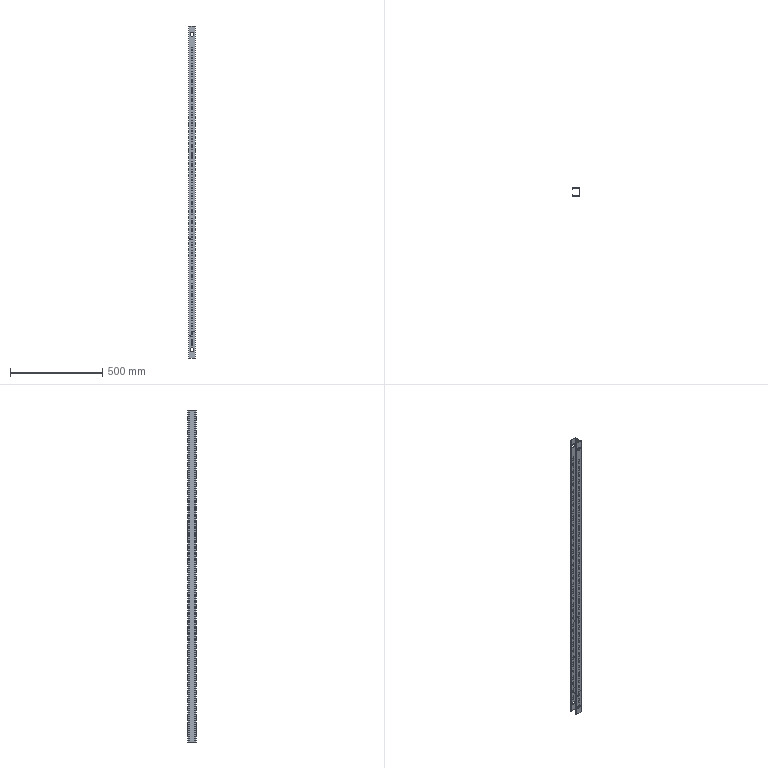Part | STEP file | SOLID | 1 solid | 654 faces | box 37 x 45 x 1797 mm | volume 330738 mm3 | cylinder 328 | plane 326 | commonest cylinder face diameters 6.5 x150 3 x148 20 x8 3.3 x6 0.4 x4 2 x4